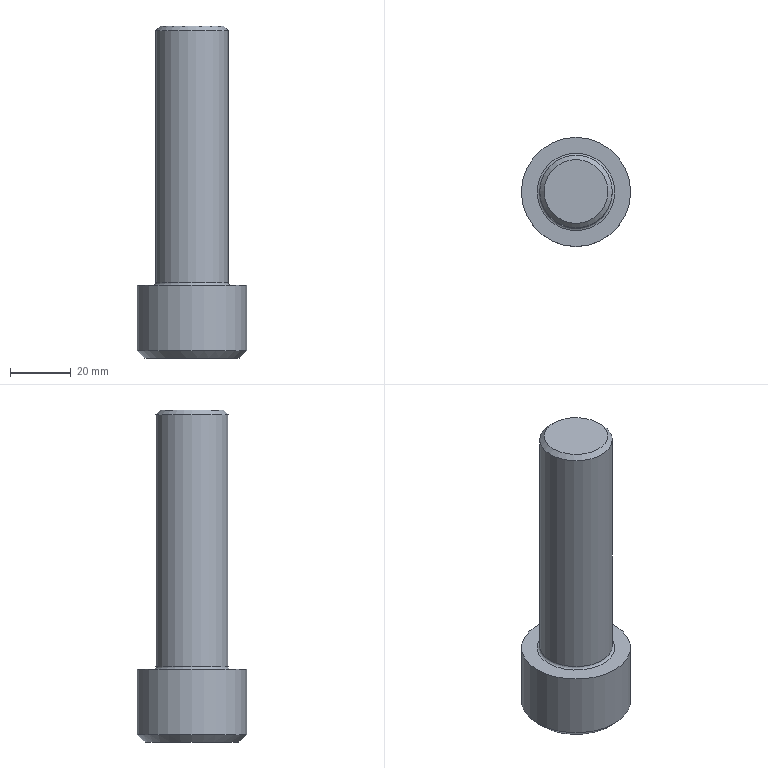Part | STEP file | solid 9 | 1 solid | 21 faces | box 36 x 36 x 109.5 mm | volume 58958 mm3 | plane 10 | sphere 6 | cylinder 2 | cone 2 | torus 1 | commonest cylinder face diameters 24 x1 36 x1